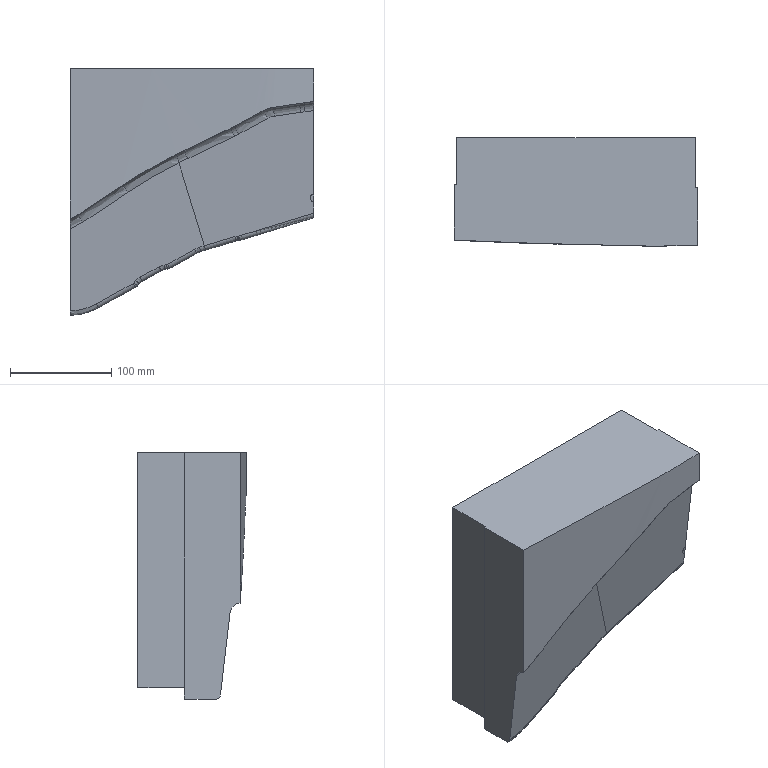Part | NX | features solid 2 | 1 solid | 96 faces | box 240.001 x 106.93 x 243.634 mm | volume 4284192 mm3 | spline 83 | plane 13